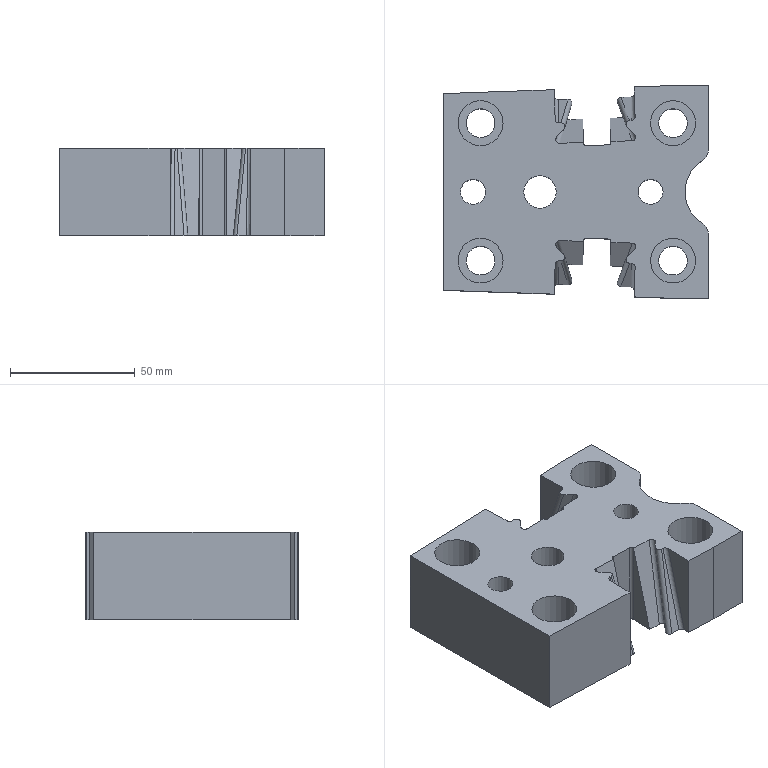Part | NX | features DIE-75 2 | 1 solid | 69 faces | box 106 x 85 x 35 mm | volume 226118 mm3 | plane 38 | cylinder 31 | commonest cylinder face diameters 3 x12 18 x5 2 x4 10 x4 11.5 x4 13 x1